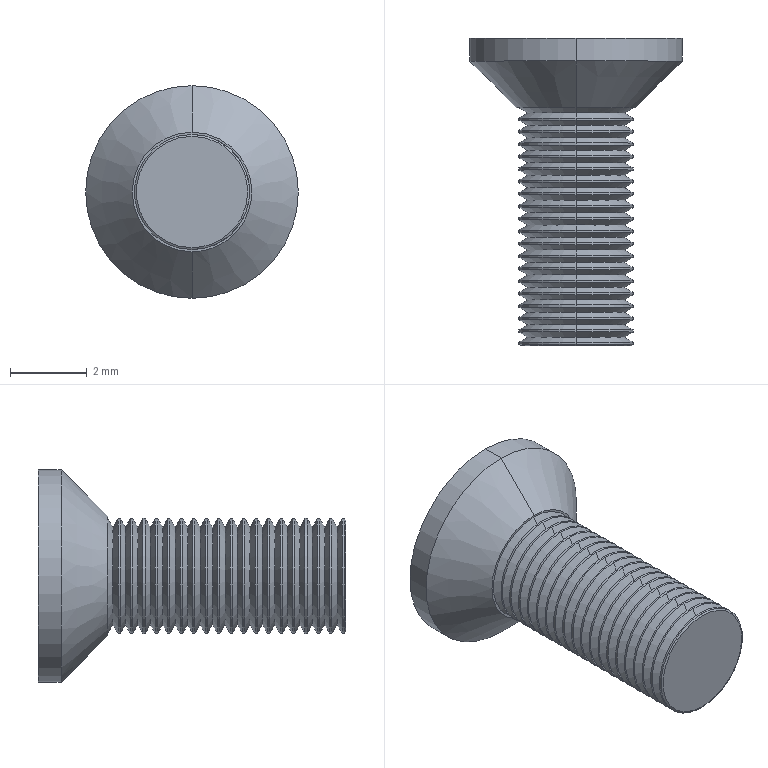Part | SolidWorks | features BaseBody 1 | 1 solid | 137 faces | box 5.54 x 8 x 5.54 mm | volume 66.538 mm3 | cone 82 | cylinder 40 | plane 15 | commonest cylinder face diameters 3 x38 5.54 x2